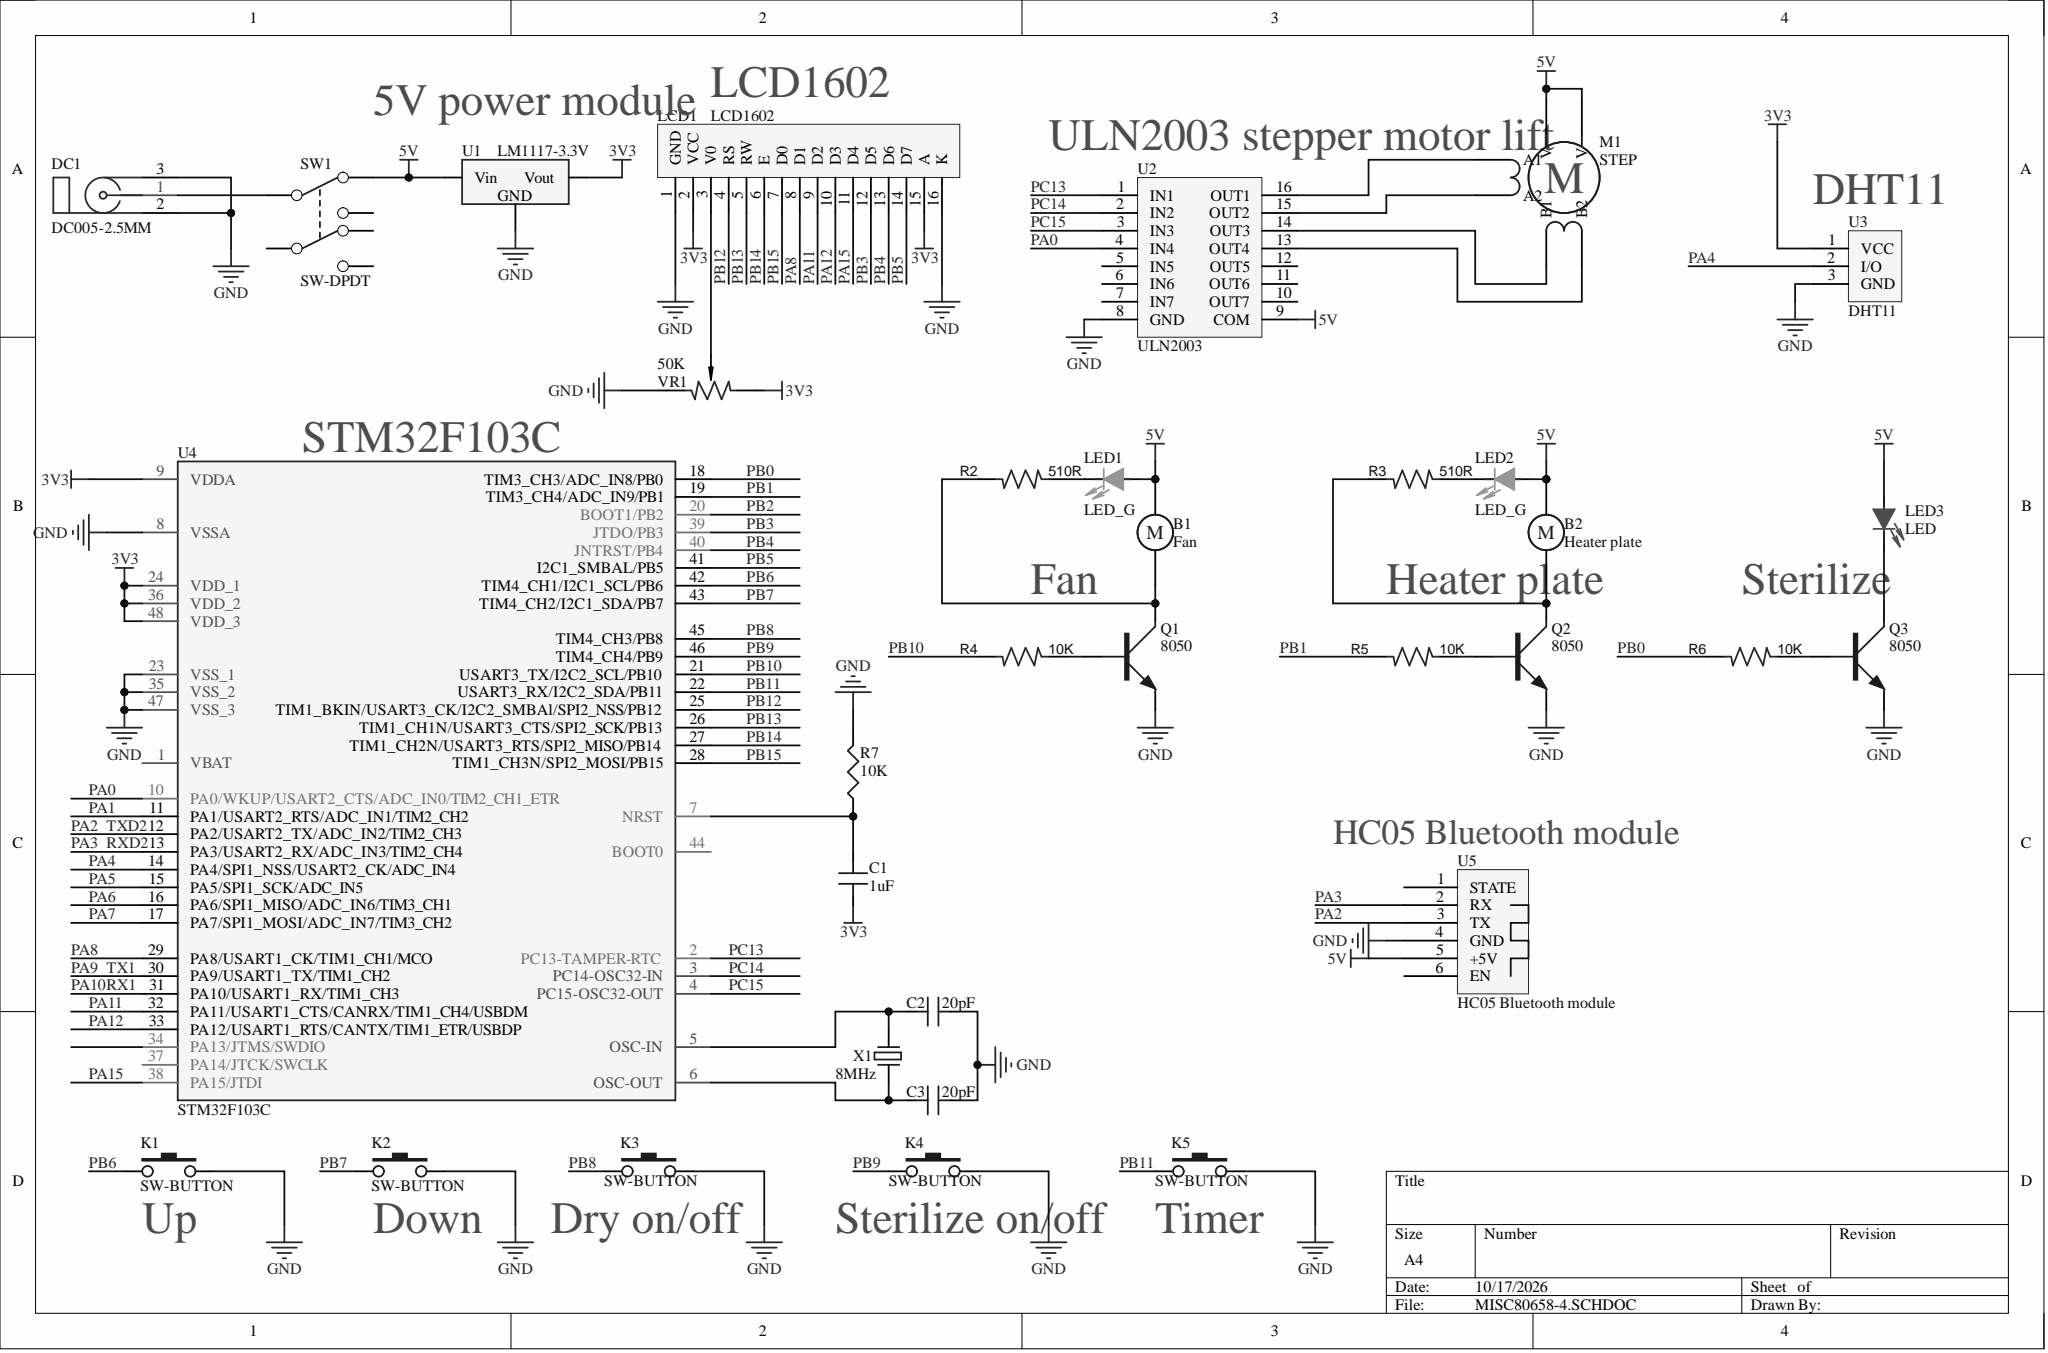Circuit board | Altium Designer | 33 parts | 46 nets
Bill of materials:
Comment,Description,Designator,Footprint,LibRef,Quantity
"Fan","5V fan","B1","RB5-10.5","Motor","1"
"Heater plate","Heater plate","B2","RB5-10.5","Motor","1"
"1uF","Chip capacitor","C1","C 0805_L","CAP","1"
"20pF","Chip capacitor","C2, C3","C 0805_L","CAP","2"
"DC005-2.5MM","","DC1","DC-005","DC005-2.5MM","1"
"SW-BUTTON","Tact switch","K1, K2, K3, K4, K5","TSW SMD-3*6*2.5","SW-BUTTON","5"
"LCD1602","LCD module","LCD1","LCD1602","LCD1602","1"
"LED_G","Green LED","LED1, LED2","LED 5MM-W","LED_G","2"
"LED","LED","LED3","LED 5MM-W","LED","1"
"STEP","Stepper motor","M1","DIP-6","MOTOR STEPPER-4_-2","1"
"8050","NPN transistor","Q1, Q2, Q3","SOT-23","NPN","3"
"510R","Resistor","R2, R3","R 0805_L","RES","2"
"10K","Resistor, [NoValue]","R4, R5, R6, R7","R 0805_L","RES, RES1","4"
"SW-DPDT","DPDT switch","SW1","KFT DIP-7X7","SW-DPDT","1"
"LM1117-3.3V","Voltage regulator circuit","U1","D2PAK","LM78xx","1"
"ULN2003","ULN2003 driver IC","U2","DIP16","ULN2003","1"
"DHT11","DHT11 temperature/humidity","U3","HDR1X3","DS18B20","1"
"STM32F103C","48-pin LQFP","U4","LQFP48 7X7","STM32F103C8T6","1"
"HC05 Bluetooth module","HC-05 Bluetooth module","U5","HDR1X6","HC-05-蓝牙模块","1"
"50K","Potentiometer","VR1","3296W","RW","1"
"8MHz","Crystal oscillator","X1","OSC 6035-2P","CRYSTAL","1"
Netlist (Protel format):
[
B1
RB5-10.5
Fan



]
[
B2
RB5-10.5
Heater plate



]
[
C1
C 0805_L
1uF



]
[
C2
C 0805_L
20pF



]
[
C3
C 0805_L
20pF



]
[
DC1
DC-005
DC005-2.5MM



]
[
K1
TSW SMD-3*6*2.5
SW-BUTTON



]
[
K2
TSW SMD-3*6*2.5
SW-BUTTON



]
[
K3
TSW SMD-3*6*2.5
SW-BUTTON



]
[
K4
TSW SMD-3*6*2.5
SW-BUTTON



]
[
K5
TSW SMD-3*6*2.5
SW-BUTTON



]
[
LCD1
LCD1602
LCD1602



]
[
LED1
LED 5MM-W
LED_G



]
[
LED2
LED 5MM-W
LED_G



]
[
LED3
LED 5MM-W
LED



]
[
M1
DIP-6
STEP



]
[
Q1
SOT-23
8050



]
[
Q2
SOT-23
8050



]
[
Q3
SOT-23
8050



]
[
R2
R 0805_L
510R



]
[
R3
R 0805_L
510R



]
[
R4
R 0805_L
10K



]
[
R5
R 0805_L
10K



]
[
R6
R 0805_L
10K



]
[
R7
R 0805_L
10K



]
[
SW1
KFT DIP-7X7
SW-DPDT



]
[
U1
D2PAK
LM1117-3.3V



]
[
U2
DIP16
ULN2003



]
[
U3
HDR1X3
DHT11



]
[
U4
LQFP48 7X7
STM32F103C



]
[
U5
HDR1X6
HC05 Bluetooth module



]
[
VR1
3296W
50K



]
[
X1
OSC 6035-2P
8MHz



]
(
PC15
U2-3
U4-4
)
(
PC14
U2-2
U4-3
)
(
PC13
U2-1
U4-2
)
(
PB15
LCD1-7
U4-28
)
(
PB14
LCD1-6
U4-27
)
(
PB13
LCD1-5
U4-26
)
(
PB12
LCD1-4
U4-25
)
(
PB11
K5-1
U4-22
)
(
PB10
R4-1
U4-21
)
(
PB9
K4-1
U4-46
)
(
PB8
K3-1
U4-45
)
(
PB7
K2-1
U4-43
)
(
PB6
K1-1
U4-42
)
(
PB5
LCD1-14
U4-41
)
(
PB4
LCD1-13
U4-40
)
(
PB3
LCD1-12
U4-39
)
(
PB1
R5-1
U4-19
)
(
PB0
R6-1
U4-18
)
(
PA15
LCD1-11
U4-38
)
(
PA12
LCD1-10
U4-33
)
(
PA11
LCD1-9
U4-32
)
(
PA8
LCD1-8
U4-29
)
(
PA4
U3-2
U4-14
)
(
PA3
U4-13
U5-2
)
(
PA2
U4-12
U5-3
)
(
PA0
U2-4
U4-10
)
(
NetQ3_B
Q3-B
R6-2
)
(
NetQ2_B
Q2-B
R5-2
)
(
NetQ1_B
Q1-B
R4-2
)
(
NetM1_6
M1-6
U2-13
)
(
NetM1_4
M1-4
U2-14
)
(
NetM1_3
M1-3
U2-15
)
(
NetM1_1
M1-1
U2-16
)
(
NetLED3_2
LED3-2
Q3-C
)
(
NetLED2_2
LED2-2
R3-2
)
(
NetLED1_2
LED1-2
R2-2
)
(
NetLCD1_3
LCD1-3
VR1-3
)
(
NetDC1_1
DC1-1
SW1-1
)
(
NetC3_1
C3-1
U4-6
X1-2
)
(
NetC2_1
C2-1
U4-5
X1-1
)
(
NetC1_2
C1-2
R7-1
U4-7
)
(
NetB2_2
B2-2
Q2-C
R3-1
)
(
NetB1_2
B1-2
Q1-C
R2-1
)
(
GND
C2-2
C3-2
DC1-2
DC1-3
K1-2
K2-2
K3-2
K4-2
K5-2
LCD1-1
LCD1-16
Q1-E
Q2-E
Q3-E
R7-2
U1-3
U2-8
U3-3
U4-8
U4-23
U4-35
U4-47
U5-4
VR1-2
)
(
5V
B1-1
B2-1
LED1-1
LED2-1
LED3-1
M1-4
M1-6
SW1-2
U1-1
U2-9
U5-5
)
(
3V3
C1-1
LCD1-2
LCD1-15
U1-2
U3-1
U4-9
U4-24
U4-36
U4-48
VR1-1
)